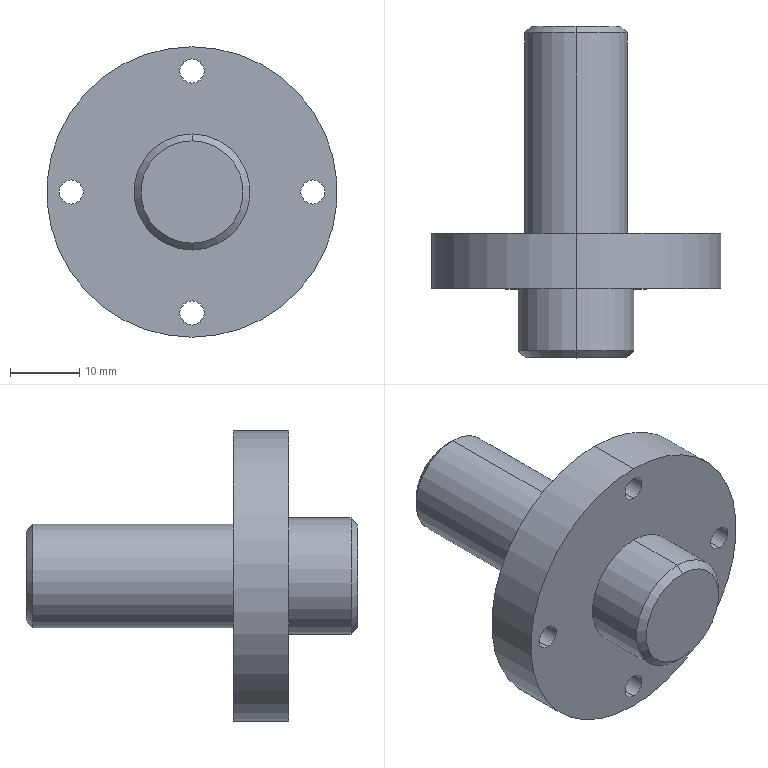Part | SolidWorks | features ICE 10, Chamfer 2, CirPattern 2, Extrusion 1 | 1 solid | 22 faces | box 42 x 48 x 42 mm | volume 18246 mm3 | cylinder 14 | cone 4 | plane 4 | commonest cylinder face diameters 3.5 x8 15 x2 16.8 x2 42 x2
STEP:
#1=CARTESIAN_POINT('',(0.,57.,-19.25));
#2=VERTEX_POINT('',#1);
#3=CARTESIAN_POINT('',(0.,57.,-15.75));
#4=VERTEX_POINT('',#3);
#5=CARTESIAN_POINT('',(0.,57.,-17.5));
#6=DIRECTION('',(0.,1.,0.));
#7=DIRECTION('',(0.,0.,1.));
#8=AXIS2_PLACEMENT_3D('',#5,#6,#7);
#9=CIRCLE('',#8,1.75);
#10=EDGE_CURVE('',#2,#4,#9,.T.);
#11=ORIENTED_EDGE('',*,*,#10,.F.);
#12=CARTESIAN_POINT('',(0.,65.,-19.25));
#13=VERTEX_POINT('',#12);
#14=CARTESIAN_POINT('',(0.,47.,-19.25));
#15=DIRECTION('',(0.,1.,0.));
#16=VECTOR('',#15,1000.);
#17=LINE('',#14,#16);
#18=EDGE_CURVE('',#2,#13,#17,.T.);
#19=ORIENTED_EDGE('',*,*,#18,.T.);
#20=CARTESIAN_POINT('',(0.,65.,-15.75));
#21=VERTEX_POINT('',#20);
#22=CARTESIAN_POINT('',(0.,65.,-17.5));
#23=DIRECTION('',(0.,1.,0.));
#24=DIRECTION('',(1.,0.,0.));
#25=AXIS2_PLACEMENT_3D('',#22,#23,#24);
#26=CIRCLE('',#25,1.75);
#27=EDGE_CURVE('',#13,#21,#26,.T.);
#28=ORIENTED_EDGE('',*,*,#27,.T.);
#29=CARTESIAN_POINT('',(0.,47.,-15.75));
#30=DIRECTION('',(0.,1.,0.));
#31=VECTOR('',#30,1000.);
#32=LINE('',#29,#31);
#33=EDGE_CURVE('',#4,#21,#32,.T.);
#34=ORIENTED_EDGE('',*,*,#33,.F.);
#35=EDGE_LOOP('',(#11,#19,#28,#34));
#36=FACE_OUTER_BOUND('',#35,.T.);
#37=CARTESIAN_POINT('',(0.,47.,-17.5));
#38=DIRECTION('',(0.,1.,0.));
#39=DIRECTION('',(0.,0.,1.));
#40=AXIS2_PLACEMENT_3D('',#37,#38,#39);
#41=CYLINDRICAL_SURFACE('',#40,1.75);
#42=ADVANCED_FACE('',(#36),#41,.F.);
#43=CARTESIAN_POINT('',(-17.5,57.,-1.75));
#44=VERTEX_POINT('',#43);
#45=CARTESIAN_POINT('',(-17.5,57.,1.75));
#46=VERTEX_POINT('',#45);
#47=CARTESIAN_POINT('',(-17.5,57.,0.));
#48=DIRECTION('',(0.,1.,0.));
#49=DIRECTION('',(0.,0.,1.));
#50=AXIS2_PLACEMENT_3D('',#47,#48,#49);
#51=CIRCLE('',#50,1.75);
#52=EDGE_CURVE('',#44,#46,#51,.T.);
#53=ORIENTED_EDGE('',*,*,#52,.F.);
#54=CARTESIAN_POINT('',(-17.5,65.,-1.75));
#55=VERTEX_POINT('',#54);
#56=CARTESIAN_POINT('',(-17.5,47.,-1.75));
#57=DIRECTION('',(0.,1.,0.));
#58=VECTOR('',#57,1000.);
#59=LINE('',#56,#58);
#60=EDGE_CURVE('',#44,#55,#59,.T.);
#61=ORIENTED_EDGE('',*,*,#60,.T.);
#62=CARTESIAN_POINT('',(-17.5,65.,1.75));
#63=VERTEX_POINT('',#62);
#64=CARTESIAN_POINT('',(-17.5,65.,0.));
#65=DIRECTION('',(0.,1.,0.));
#66=DIRECTION('',(0.,0.,-1.));
#67=AXIS2_PLACEMENT_3D('',#64,#65,#66);
#68=CIRCLE('',#67,1.75);
#69=EDGE_CURVE('',#55,#63,#68,.T.);
#70=ORIENTED_EDGE('',*,*,#69,.T.);
#71=CARTESIAN_POINT('',(-17.5,47.,1.75));
#72=DIRECTION('',(0.,1.,0.));
#73=VECTOR('',#72,1000.);
#74=LINE('',#71,#73);
#75=EDGE_CURVE('',#46,#63,#74,.T.);
#76=ORIENTED_EDGE('',*,*,#75,.F.);
#77=EDGE_LOOP('',(#53,#61,#70,#76));
#78=FACE_OUTER_BOUND('',#77,.T.);
#79=CARTESIAN_POINT('',(-17.5,47.,0.));
#80=DIRECTION('',(0.,1.,0.));
#81=DIRECTION('',(0.,0.,1.));
#82=AXIS2_PLACEMENT_3D('',#79,#80,#81);
#83=CYLINDRICAL_SURFACE('',#82,1.75);
#84=ADVANCED_FACE('',(#78),#83,.F.);
#85=CARTESIAN_POINT('',(0.,57.,15.75));
#86=VERTEX_POINT('',#85);
#87=CARTESIAN_POINT('',(0.,57.,19.25));
#88=VERTEX_POINT('',#87);
#89=CARTESIAN_POINT('',(0.,57.,17.5));
#90=DIRECTION('',(0.,1.,0.));
#91=DIRECTION('',(0.,0.,1.));
#92=AXIS2_PLACEMENT_3D('',#89,#90,#91);
#93=CIRCLE('',#92,1.75);
#94=EDGE_CURVE('',#86,#88,#93,.T.);
#95=ORIENTED_EDGE('',*,*,#94,.F.);
#96=CARTESIAN_POINT('',(0.,65.,15.75));
#97=VERTEX_POINT('',#96);
#98=CARTESIAN_POINT('',(0.,47.,15.75));
#99=DIRECTION('',(0.,1.,0.));
#100=VECTOR('',#99,1000.);
#101=LINE('',#98,#100);
#102=EDGE_CURVE('',#86,#97,#101,.T.);
#103=ORIENTED_EDGE('',*,*,#102,.T.);
#104=CARTESIAN_POINT('',(0.,65.,19.25));
#105=VERTEX_POINT('',#104);
#106=CARTESIAN_POINT('',(0.,65.,17.5));
#107=DIRECTION('',(0.,1.,0.));
#108=DIRECTION('',(-1.,0.,0.));
#109=AXIS2_PLACEMENT_3D('',#106,#107,#108);
#110=CIRCLE('',#109,1.75);
#111=EDGE_CURVE('',#97,#105,#110,.T.);
#112=ORIENTED_EDGE('',*,*,#111,.T.);
#113=CARTESIAN_POINT('',(0.,47.,19.25));
#114=DIRECTION('',(0.,1.,0.));
#115=VECTOR('',#114,1000.);
#116=LINE('',#113,#115);
#117=EDGE_CURVE('',#88,#105,#116,.T.);
#118=ORIENTED_EDGE('',*,*,#117,.F.);
#119=EDGE_LOOP('',(#95,#103,#112,#118));
#120=FACE_OUTER_BOUND('',#119,.T.);
#121=CARTESIAN_POINT('',(0.,47.,17.5));
#122=DIRECTION('',(0.,1.,0.));
#123=DIRECTION('',(0.,0.,1.));
#124=AXIS2_PLACEMENT_3D('',#121,#122,#123);
#125=CYLINDRICAL_SURFACE('',#124,1.75);
#126=ADVANCED_FACE('',(#120),#125,.F.);
#127=CARTESIAN_POINT('',(17.5,57.,-1.75));
#128=VERTEX_POINT('',#127);
#129=CARTESIAN_POINT('',(17.5,57.,1.75));
#130=VERTEX_POINT('',#129);
#131=CARTESIAN_POINT('',(17.5,57.,0.));
#132=DIRECTION('',(0.,1.,0.));
#133=DIRECTION('',(0.,0.,1.));
#134=AXIS2_PLACEMENT_3D('',#131,#132,#133);
#135=CIRCLE('',#134,1.75);
#136=EDGE_CURVE('',#128,#130,#135,.T.);
#137=ORIENTED_EDGE('',*,*,#136,.F.);
#138=CARTESIAN_POINT('',(17.5,65.,-1.75));
#139=VERTEX_POINT('',#138);
#140=CARTESIAN_POINT('',(17.5,47.,-1.75));
#141=DIRECTION('',(0.,1.,0.));
#142=VECTOR('',#141,1000.);
#143=LINE('',#140,#142);
#144=EDGE_CURVE('',#128,#139,#143,.T.);
#145=ORIENTED_EDGE('',*,*,#144,.T.);
#146=CARTESIAN_POINT('',(17.5,65.,1.75));
#147=VERTEX_POINT('',#146);
#148=CARTESIAN_POINT('',(17.5,65.,0.));
#149=DIRECTION('',(0.,1.,0.));
#150=DIRECTION('',(0.,0.,1.));
#151=AXIS2_PLACEMENT_3D('',#148,#149,#150);
#152=CIRCLE('',#151,1.75);
#153=EDGE_CURVE('',#139,#147,#152,.T.);
#154=ORIENTED_EDGE('',*,*,#153,.T.);
#155=CARTESIAN_POINT('',(17.5,47.,1.75));
#156=DIRECTION('',(0.,1.,0.));
#157=VECTOR('',#156,1000.);
#158=LINE('',#155,#157);
#159=EDGE_CURVE('',#130,#147,#158,.T.);
#160=ORIENTED_EDGE('',*,*,#159,.F.);
#161=EDGE_LOOP('',(#137,#145,#154,#160));
#162=FACE_OUTER_BOUND('',#161,.T.);
#163=CARTESIAN_POINT('',(17.5,47.,0.));
#164=DIRECTION('',(0.,1.,0.));
#165=DIRECTION('',(0.,0.,1.));
#166=AXIS2_PLACEMENT_3D('',#163,#164,#165);
#167=CYLINDRICAL_SURFACE('',#166,1.75);
#168=ADVANCED_FACE('',(#162),#167,.F.);
#169=CARTESIAN_POINT('',(0.,47.,-7.4));
#170=VERTEX_POINT('',#169);
#171=CARTESIAN_POINT('',(0.,47.,7.4));
#172=VERTEX_POINT('',#171);
#173=CARTESIAN_POINT('',(0.,47.,0.));
#174=DIRECTION('',(0.,-1.,0.));
#175=DIRECTION('',(0.,0.,-1.));
#176=AXIS2_PLACEMENT_3D('',#173,#174,#175);
#177=CIRCLE('',#176,7.4);
#178=EDGE_CURVE('',#170,#172,#177,.T.);
#179=ORIENTED_EDGE('',*,*,#178,.F.);
#180=CARTESIAN_POINT('',(0.,48.,-8.4));
#181=VERTEX_POINT('',#180);
#182=CARTESIAN_POINT('',(0.,47.,-7.4));
#183=DIRECTION('',(0.,0.7071,-0.7071));
#184=VECTOR('',#183,1000.);
#185=LINE('',#182,#184);
#186=EDGE_CURVE('',#170,#181,#185,.T.);
#187=ORIENTED_EDGE('',*,*,#186,.T.);
#188=CARTESIAN_POINT('',(0.,48.,8.4));
#189=VERTEX_POINT('',#188);
#190=CARTESIAN_POINT('',(0.,48.,0.));
#191=DIRECTION('',(0.,1.,0.));
#192=DIRECTION('',(0.,0.,-1.));
#193=AXIS2_PLACEMENT_3D('',#190,#191,#192);
#194=CIRCLE('',#193,8.4);
#195=EDGE_CURVE('',#189,#181,#194,.T.);
#196=ORIENTED_EDGE('',*,*,#195,.F.);
#197=CARTESIAN_POINT('',(0.,47.,7.4));
#198=DIRECTION('',(0.,0.7071,0.7071));
#199=VECTOR('',#198,1000.);
#200=LINE('',#197,#199);
#201=EDGE_CURVE('',#172,#189,#200,.T.);
#202=ORIENTED_EDGE('',*,*,#201,.F.);
#203=EDGE_LOOP('',(#179,#187,#196,#202));
#204=FACE_OUTER_BOUND('',#203,.T.);
#205=CARTESIAN_POINT('',(0.,47.,0.));
#206=DIRECTION('',(0.,1.,0.));
#207=DIRECTION('',(0.,0.,1.));
#208=AXIS2_PLACEMENT_3D('',#205,#206,#207);
#209=CONICAL_SURFACE('',#208,7.4,0.7854);
#210=ADVANCED_FACE('',(#204),#209,.T.);
#211=CARTESIAN_POINT('',(0.,95.,6.5));
#212=VERTEX_POINT('',#211);
#213=CARTESIAN_POINT('',(0.,95.,-6.5));
#214=VERTEX_POINT('',#213);
#215=CARTESIAN_POINT('',(0.,95.,0.));
#216=DIRECTION('',(0.,1.,0.));
#217=DIRECTION('',(0.,0.,1.));
#218=AXIS2_PLACEMENT_3D('',#215,#216,#217);
#219=CIRCLE('',#218,6.5);
#220=EDGE_CURVE('',#212,#214,#219,.T.);
#221=ORIENTED_EDGE('',*,*,#220,.F.);
#222=CARTESIAN_POINT('',(0.,94.,7.5));
#223=VERTEX_POINT('',#222);
#224=CARTESIAN_POINT('',(0.,95.,6.5));
#225=DIRECTION('',(0.,-0.7071,0.7071));
#226=VECTOR('',#225,1000.);
#227=LINE('',#224,#226);
#228=EDGE_CURVE('',#212,#223,#227,.T.);
#229=ORIENTED_EDGE('',*,*,#228,.T.);
#230=CARTESIAN_POINT('',(0.,94.,-7.5));
#231=VERTEX_POINT('',#230);
#232=CARTESIAN_POINT('',(0.,94.,0.));
#233=DIRECTION('',(0.,-1.,0.));
#234=DIRECTION('',(0.,0.,1.));
#235=AXIS2_PLACEMENT_3D('',#232,#233,#234);
#236=CIRCLE('',#235,7.5);
#237=EDGE_CURVE('',#231,#223,#236,.T.);
#238=ORIENTED_EDGE('',*,*,#237,.F.);
#239=CARTESIAN_POINT('',(0.,95.,-6.5));
#240=DIRECTION('',(0.,-0.7071,-0.7071));
#241=VECTOR('',#240,1000.);
#242=LINE('',#239,#241);
#243=EDGE_CURVE('',#214,#231,#242,.T.);
#244=ORIENTED_EDGE('',*,*,#243,.F.);
#245=EDGE_LOOP('',(#221,#229,#238,#244));
#246=FACE_OUTER_BOUND('',#245,.T.);
#247=CARTESIAN_POINT('',(0.,95.,0.));
#248=DIRECTION('',(0.,-1.,0.));
#249=DIRECTION('',(0.,0.,-1.));
#250=AXIS2_PLACEMENT_3D('',#247,#248,#249);
#251=CONICAL_SURFACE('',#250,6.5,0.7854);
#252=ADVANCED_FACE('',(#246),#251,.T.);
#253=ORIENTED_EDGE('',*,*,#195,.T.);
#254=CARTESIAN_POINT('',(0.,57.,-8.4));
#255=VERTEX_POINT('',#254);
#256=CARTESIAN_POINT('',(0.,47.,-8.4));
#257=DIRECTION('',(0.,1.,0.));
#258=VECTOR('',#257,1000.);
#259=LINE('',#256,#258);
#260=EDGE_CURVE('',#181,#255,#259,.T.);
#261=ORIENTED_EDGE('',*,*,#260,.T.);
#262=CARTESIAN_POINT('',(0.,57.,8.4));
#263=VERTEX_POINT('',#262);
#264=CARTESIAN_POINT('',(0.,57.,0.));
#265=DIRECTION('',(0.,-1.,0.));
#266=DIRECTION('',(0.,0.,1.));
#267=AXIS2_PLACEMENT_3D('',#264,#265,#266);
#268=CIRCLE('',#267,8.4);
#269=EDGE_CURVE('',#255,#263,#268,.T.);
#270=ORIENTED_EDGE('',*,*,#269,.T.);
#271=CARTESIAN_POINT('',(0.,47.,8.4));
#272=DIRECTION('',(0.,1.,0.));
#273=VECTOR('',#272,1000.);
#274=LINE('',#271,#273);
#275=EDGE_CURVE('',#189,#263,#274,.T.);
#276=ORIENTED_EDGE('',*,*,#275,.F.);
#277=EDGE_LOOP('',(#253,#261,#270,#276));
#278=FACE_OUTER_BOUND('',#277,.T.);
#279=CARTESIAN_POINT('',(0.,47.,0.));
#280=DIRECTION('',(0.,1.,0.));
#281=DIRECTION('',(0.,0.,1.));
#282=AXIS2_PLACEMENT_3D('',#279,#280,#281);
#283=CYLINDRICAL_SURFACE('',#282,8.4);
#284=ADVANCED_FACE('',(#278),#283,.T.);
#285=ORIENTED_EDGE('',*,*,#237,.T.);
#286=CARTESIAN_POINT('',(0.,65.,7.5));
#287=VERTEX_POINT('',#286);
#288=CARTESIAN_POINT('',(0.,95.,7.5));
#289=DIRECTION('',(0.,-1.,0.));
#290=VECTOR('',#289,1000.);
#291=LINE('',#288,#290);
#292=EDGE_CURVE('',#223,#287,#291,.T.);
#293=ORIENTED_EDGE('',*,*,#292,.T.);
#294=CARTESIAN_POINT('',(0.,65.,-7.5));
#295=VERTEX_POINT('',#294);
#296=CARTESIAN_POINT('',(0.,65.,0.));
#297=DIRECTION('',(0.,1.,0.));
#298=DIRECTION('',(0.,0.,1.));
#299=AXIS2_PLACEMENT_3D('',#296,#297,#298);
#300=CIRCLE('',#299,7.5);
#301=EDGE_CURVE('',#287,#295,#300,.T.);
#302=ORIENTED_EDGE('',*,*,#301,.T.);
#303=CARTESIAN_POINT('',(0.,95.,-7.5));
#304=DIRECTION('',(0.,-1.,0.));
#305=VECTOR('',#304,1000.);
#306=LINE('',#303,#305);
#307=EDGE_CURVE('',#231,#295,#306,.T.);
#308=ORIENTED_EDGE('',*,*,#307,.F.);
#309=EDGE_LOOP('',(#285,#293,#302,#308));
#310=FACE_OUTER_BOUND('',#309,.T.);
#311=CARTESIAN_POINT('',(0.,95.,0.));
#312=DIRECTION('',(0.,-1.,0.));
#313=DIRECTION('',(0.,0.,-1.));
#314=AXIS2_PLACEMENT_3D('',#311,#312,#313);
#315=CYLINDRICAL_SURFACE('',#314,7.5);
#316=ADVANCED_FACE('',(#310),#315,.T.);
#317=CARTESIAN_POINT('',(0.,57.,21.));
#318=VERTEX_POINT('',#317);
#319=CARTESIAN_POINT('',(0.,57.,-21.));
#320=VERTEX_POINT('',#319);
#321=CARTESIAN_POINT('',(0.,57.,0.));
#322=DIRECTION('',(0.,1.,0.));
#323=DIRECTION('',(0.,0.,1.));
#324=AXIS2_PLACEMENT_3D('',#321,#322,#323);
#325=CIRCLE('',#324,21.);
#326=EDGE_CURVE('',#318,#320,#325,.T.);
#327=ORIENTED_EDGE('',*,*,#326,.T.);
#328=CARTESIAN_POINT('',(0.,65.,-21.));
#329=VERTEX_POINT('',#328);
#330=CARTESIAN_POINT('',(0.,57.,-21.));
#331=DIRECTION('',(0.,1.,0.));
#332=VECTOR('',#331,1000.);
#333=LINE('',#330,#332);
#334=EDGE_CURVE('',#320,#329,#333,.T.);
#335=ORIENTED_EDGE('',*,*,#334,.T.);
#336=CARTESIAN_POINT('',(0.,65.,21.));
#337=VERTEX_POINT('',#336);
#338=CARTESIAN_POINT('',(0.,65.,0.));
#339=DIRECTION('',(0.,1.,0.));
#340=DIRECTION('',(0.,0.,1.));
#341=AXIS2_PLACEMENT_3D('',#338,#339,#340);
#342=CIRCLE('',#341,21.);
#343=EDGE_CURVE('',#337,#329,#342,.T.);
#344=ORIENTED_EDGE('',*,*,#343,.F.);
#345=CARTESIAN_POINT('',(0.,57.,21.));
#346=DIRECTION('',(0.,1.,0.));
#347=VECTOR('',#346,1000.);
#348=LINE('',#345,#347);
#349=EDGE_CURVE('',#318,#337,#348,.T.);
#350=ORIENTED_EDGE('',*,*,#349,.F.);
#351=EDGE_LOOP('',(#327,#335,#344,#350));
#352=FACE_OUTER_BOUND('',#351,.T.);
#353=CARTESIAN_POINT('',(0.,57.,0.));
#354=DIRECTION('',(0.,1.,0.));
#355=DIRECTION('',(0.,0.,1.));
#356=AXIS2_PLACEMENT_3D('',#353,#354,#355);
#357=CYLINDRICAL_SURFACE('',#356,21.);
#358=ADVANCED_FACE('',(#352),#357,.T.);
#359=CARTESIAN_POINT('',(0.,57.,-17.5));
#360=DIRECTION('',(0.,1.,0.));
#361=DIRECTION('',(0.,0.,1.));
#362=AXIS2_PLACEMENT_3D('',#359,#360,#361);
#363=CIRCLE('',#362,1.75);
#364=EDGE_CURVE('',#4,#2,#363,.T.);
#365=ORIENTED_EDGE('',*,*,#364,.T.);
#366=ORIENTED_EDGE('',*,*,#10,.T.);
#367=EDGE_LOOP('',(#365,#366));
#368=FACE_BOUND('',#367,.T.);
#369=CARTESIAN_POINT('',(-17.5,57.,0.));
#370=DIRECTION('',(0.,1.,0.));
#371=DIRECTION('',(0.,0.,1.));
#372=AXIS2_PLACEMENT_3D('',#369,#370,#371);
#373=CIRCLE('',#372,1.75);
#374=EDGE_CURVE('',#46,#44,#373,.T.);
#375=ORIENTED_EDGE('',*,*,#374,.T.);
#376=ORIENTED_EDGE('',*,*,#52,.T.);
#377=EDGE_LOOP('',(#375,#376));
#378=FACE_BOUND('',#377,.T.);
#379=CARTESIAN_POINT('',(0.,57.,17.5));
#380=DIRECTION('',(0.,1.,0.));
#381=DIRECTION('',(0.,0.,1.));
#382=AXIS2_PLACEMENT_3D('',#379,#380,#381);
#383=CIRCLE('',#382,1.75);
#384=EDGE_CURVE('',#88,#86,#383,.T.);
#385=ORIENTED_EDGE('',*,*,#384,.T.);
#386=ORIENTED_EDGE('',*,*,#94,.T.);
#387=EDGE_LOOP('',(#385,#386));
#388=FACE_BOUND('',#387,.T.);
#389=CARTESIAN_POINT('',(17.5,57.,0.));
#390=DIRECTION('',(0.,1.,0.));
#391=DIRECTION('',(0.,0.,1.));
#392=AXIS2_PLACEMENT_3D('',#389,#390,#391);
#393=CIRCLE('',#392,1.75);
#394=EDGE_CURVE('',#130,#128,#393,.T.);
#395=ORIENTED_EDGE('',*,*,#394,.T.);
#396=ORIENTED_EDGE('',*,*,#136,.T.);
#397=EDGE_LOOP('',(#395,#396));
#398=FACE_BOUND('',#397,.T.);
#399=ORIENTED_EDGE('',*,*,#326,.F.);
#400=CARTESIAN_POINT('',(0.,57.,0.));
#401=DIRECTION('',(0.,1.,0.));
#402=DIRECTION('',(0.,0.,1.));
#403=AXIS2_PLACEMENT_3D('',#400,#401,#402);
#404=CIRCLE('',#403,21.);
#405=EDGE_CURVE('',#320,#318,#404,.T.);
#406=ORIENTED_EDGE('',*,*,#405,.F.);
#407=EDGE_LOOP('',(#399,#406));
#408=FACE_OUTER_BOUND('',#407,.T.);
#409=CARTESIAN_POINT('',(0.,57.,0.));
#410=DIRECTION('',(0.,-1.,0.));
#411=DIRECTION('',(0.,0.,1.));
#412=AXIS2_PLACEMENT_3D('',#409,#410,#411);
#413=CIRCLE('',#412,8.4);
#414=EDGE_CURVE('',#263,#255,#413,.T.);
#415=ORIENTED_EDGE('',*,*,#414,.F.);
#416=ORIENTED_EDGE('',*,*,#269,.F.);
#417=EDGE_LOOP('',(#415,#416));
#418=FACE_BOUND('',#417,.T.);
#419=CARTESIAN_POINT('',(0.,57.,0.));
#420=DIRECTION('',(0.,1.,0.));
#421=DIRECTION('',(0.,0.,1.));
#422=AXIS2_PLACEMENT_3D('',#419,#420,#421);
#423=PLANE('',#422);
#424=ADVANCED_FACE('',(#368,#378,#388,#398,#408,#418),#423,.F.);
#425=ORIENTED_EDGE('',*,*,#334,.F.);
#426=ORIENTED_EDGE('',*,*,#405,.T.);
#427=ORIENTED_EDGE('',*,*,#349,.T.);
#428=CARTESIAN_POINT('',(0.,65.,0.));
#429=DIRECTION('',(0.,1.,0.));
#430=DIRECTION('',(0.,0.,1.));
#431=AXIS2_PLACEMENT_3D('',#428,#429,#430);
#432=CIRCLE('',#431,21.);
#433=EDGE_CURVE('',#329,#337,#432,.T.);
#434=ORIENTED_EDGE('',*,*,#433,.F.);
#435=EDGE_LOOP('',(#425,#426,#427,#434));
#436=FACE_OUTER_BOUND('',#435,.T.);
#437=CARTESIAN_POINT('',(0.,57.,0.));
#438=DIRECTION('',(0.,1.,0.));
#439=DIRECTION('',(0.,0.,1.));
#440=AXIS2_PLACEMENT_3D('',#437,#438,#439);
#441=CYLINDRICAL_SURFACE('',#440,21.);
#442=ADVANCED_FACE('',(#436),#441,.T.);
#443=CARTESIAN_POINT('',(0.,95.,0.));
#444=DIRECTION('',(0.,1.,0.));
#445=DIRECTION('',(0.,0.,1.));
#446=AXIS2_PLACEMENT_3D('',#443,#444,#445);
#447=CIRCLE('',#446,6.5);
#448=EDGE_CURVE('',#214,#212,#447,.T.);
#449=ORIENTED_EDGE('',*,*,#448,.T.);
#450=ORIENTED_EDGE('',*,*,#220,.T.);
#451=EDGE_LOOP('',(#449,#450));
#452=FACE_OUTER_BOUND('',#451,.T.);
#453=CARTESIAN_POINT('',(0.,95.,0.));
#454=DIRECTION('',(0.,1.,0.));
#455=DIRECTION('',(0.,0.,1.));
#456=AXIS2_PLACEMENT_3D('',#453,#454,#455);
#457=PLANE('',#456);
#458=ADVANCED_FACE('',(#452),#457,.T.);
#459=ORIENTED_EDGE('',*,*,#292,.F.);
#460=CARTESIAN_POINT('',(0.,94.,0.));
#461=DIRECTION('',(0.,-1.,0.));
#462=DIRECTION('',(0.,0.,1.));
#463=AXIS2_PLACEMENT_3D('',#460,#461,#462);
#464=CIRCLE('',#463,7.5);
#465=EDGE_CURVE('',#223,#231,#464,.T.);
#466=ORIENTED_EDGE('',*,*,#465,.T.);
#467=ORIENTED_EDGE('',*,*,#307,.T.);
#468=CARTESIAN_POINT('',(0.,65.,0.));
#469=DIRECTION('',(0.,1.,0.));
#470=DIRECTION('',(0.,0.,1.));
#471=AXIS2_PLACEMENT_3D('',#468,#469,#470);
#472=CIRCLE('',#471,7.5);
#473=EDGE_CURVE('',#295,#287,#472,.T.);
#474=ORIENTED_EDGE('',*,*,#473,.T.);
#475=EDGE_LOOP('',(#459,#466,#467,#474));
#476=FACE_OUTER_BOUND('',#475,.T.);
#477=CARTESIAN_POINT('',(0.,95.,0.));
#478=DIRECTION('',(0.,-1.,0.));
#479=DIRECTION('',(0.,0.,-1.));
#480=AXIS2_PLACEMENT_3D('',#477,#478,#479);
#481=CYLINDRICAL_SURFACE('',#480,7.5);
#482=ADVANCED_FACE('',(#476),#481,.T.);
#483=CARTESIAN_POINT('',(0.,65.,-17.5));
#484=DIRECTION('',(0.,1.,0.));
#485=DIRECTION('',(1.,0.,0.));
#486=AXIS2_PLACEMENT_3D('',#483,#484,#485);
#487=CIRCLE('',#486,1.75);
#488=EDGE_CURVE('',#21,#13,#487,.T.);
#489=ORIENTED_EDGE('',*,*,#488,.F.);
#490=ORIENTED_EDGE('',*,*,#27,.F.);
#491=EDGE_LOOP('',(#489,#490));
#492=FACE_BOUND('',#491,.T.);
#493=CARTESIAN_POINT('',(-17.5,65.,0.));
#494=DIRECTION('',(0.,1.,0.));
#495=DIRECTION('',(0.,0.,-1.));
#496=AXIS2_PLACEMENT_3D('',#493,#494,#495);
#497=CIRCLE('',#496,1.75);
#498=EDGE_CURVE('',#63,#55,#497,.T.);
#499=ORIENTED_EDGE('',*,*,#498,.F.);
#500=ORIENTED_EDGE('',*,*,#69,.F.);
#501=EDGE_LOOP('',(#499,#500));
#502=FACE_BOUND('',#501,.T.);
#503=CARTESIAN_POINT('',(0.,65.,17.5));
#504=DIRECTION('',(0.,1.,0.));
#505=DIRECTION('',(-1.,0.,0.));
#506=AXIS2_PLACEMENT_3D('',#503,#504,#505);
#507=CIRCLE('',#506,1.75);
#508=EDGE_CURVE('',#105,#97,#507,.T.);
#509=ORIENTED_EDGE('',*,*,#508,.F.);
#510=ORIENTED_EDGE('',*,*,#111,.F.);
#511=EDGE_LOOP('',(#509,#510));
#512=FACE_BOUND('',#511,.T.);
#513=CARTESIAN_POINT('',(17.5,65.,0.));
#514=DIRECTION('',(0.,1.,0.));
#515=DIRECTION('',(0.,0.,1.));
#516=AXIS2_PLACEMENT_3D('',#513,#514,#515);
#517=CIRCLE('',#516,1.75);
#518=EDGE_CURVE('',#147,#139,#517,.T.);
#519=ORIENTED_EDGE('',*,*,#518,.F.);
#520=ORIENTED_EDGE('',*,*,#153,.F.);
#521=EDGE_LOOP('',(#519,#520));
#522=FACE_BOUND('',#521,.T.);
#523=ORIENTED_EDGE('',*,*,#473,.F.);
#524=ORIENTED_EDGE('',*,*,#301,.F.);
#525=EDGE_LOOP('',(#523,#524));
#526=FACE_BOUND('',#525,.T.);
#527=ORIENTED_EDGE('',*,*,#343,.T.);
#528=ORIENTED_EDGE('',*,*,#433,.T.);
#529=EDGE_LOOP('',(#527,#528));
#530=FACE_OUTER_BOUND('',#529,.T.);
#531=CARTESIAN_POINT('',(0.,65.,0.));
#532=DIRECTION('',(0.,1.,0.));
#533=DIRECTION('',(0.,0.,1.));
#534=AXIS2_PLACEMENT_3D('',#531,#532,#533);
#535=PLANE('',#534);
#536=ADVANCED_FACE('',(#492,#502,#512,#522,#526,#530),#535,.T.);
#537=ORIENTED_EDGE('',*,*,#260,.F.);
#538=CARTESIAN_POINT('',(0.,48.,0.));
#539=DIRECTION('',(0.,1.,0.));
#540=DIRECTION('',(0.,0.,-1.));
#541=AXIS2_PLACEMENT_3D('',#538,#539,#540);
#542=CIRCLE('',#541,8.4);
#543=EDGE_CURVE('',#181,#189,#542,.T.);
#544=ORIENTED_EDGE('',*,*,#543,.T.);
#545=ORIENTED_EDGE('',*,*,#275,.T.);
#546=ORIENTED_EDGE('',*,*,#414,.T.);
#547=EDGE_LOOP('',(#537,#544,#545,#546));
#548=FACE_OUTER_BOUND('',#547,.T.);
#549=CARTESIAN_POINT('',(0.,47.,0.));
#550=DIRECTION('',(0.,1.,0.));
#551=DIRECTION('',(0.,0.,1.));
#552=AXIS2_PLACEMENT_3D('',#549,#550,#551);
#553=CYLINDRICAL_SURFACE('',#552,8.4);
#554=ADVANCED_FACE('',(#548),#553,.T.);
#555=CARTESIAN_POINT('',(0.,47.,0.));
#556=DIRECTION('',(0.,-1.,0.));
#557=DIRECTION('',(0.,0.,-1.));
#558=AXIS2_PLACEMENT_3D('',#555,#556,#557);
#559=CIRCLE('',#558,7.4);
#560=EDGE_CURVE('',#172,#170,#559,.T.);
#561=ORIENTED_EDGE('',*,*,#560,.T.);
#562=ORIENTED_EDGE('',*,*,#178,.T.);
#563=EDGE_LOOP('',(#561,#562));
#564=FACE_OUTER_BOUND('',#563,.T.);
#565=CARTESIAN_POINT('',(0.,47.,0.));
#566=DIRECTION('',(0.,-1.,0.));
#567=DIRECTION('',(0.,0.,-1.));
#568=AXIS2_PLACEMENT_3D('',#565,#566,#567);
#569=PLANE('',#568);
#570=ADVANCED_FACE('',(#564),#569,.T.);
#571=ORIENTED_EDGE('',*,*,#228,.F.);
#572=ORIENTED_EDGE('',*,*,#448,.F.);
#573=ORIENTED_EDGE('',*,*,#243,.T.);
#574=ORIENTED_EDGE('',*,*,#465,.F.);
#575=EDGE_LOOP('',(#571,#572,#573,#574));
#576=FACE_OUTER_BOUND('',#575,.T.);
#577=CARTESIAN_POINT('',(0.,95.,0.));
#578=DIRECTION('',(0.,-1.,0.));
#579=DIRECTION('',(0.,0.,-1.));
#580=AXIS2_PLACEMENT_3D('',#577,#578,#579);
#581=CONICAL_SURFACE('',#580,6.5,0.7854);
#582=ADVANCED_FACE('',(#576),#581,.T.);
#583=ORIENTED_EDGE('',*,*,#186,.F.);
#584=ORIENTED_EDGE('',*,*,#560,.F.);
#585=ORIENTED_EDGE('',*,*,#201,.T.);
#586=ORIENTED_EDGE('',*,*,#543,.F.);
#587=EDGE_LOOP('',(#583,#584,#585,#586));
#588=FACE_OUTER_BOUND('',#587,.T.);
#589=CARTESIAN_POINT('',(0.,47.,0.));
#590=DIRECTION('',(0.,1.,0.));
#591=DIRECTION('',(0.,0.,1.));
#592=AXIS2_PLACEMENT_3D('',#589,#590,#591);
#593=CONICAL_SURFACE('',#592,7.4,0.7854);
#594=ADVANCED_FACE('',(#588),#593,.T.);
#595=ORIENTED_EDGE('',*,*,#144,.F.);
#596=ORIENTED_EDGE('',*,*,#394,.F.);
#597=ORIENTED_EDGE('',*,*,#159,.T.);
#598=ORIENTED_EDGE('',*,*,#518,.T.);
#599=EDGE_LOOP('',(#595,#596,#597,#598));
#600=FACE_OUTER_BOUND('',#599,.T.);
#601=CARTESIAN_POINT('',(17.5,47.,0.));
#602=DIRECTION('',(0.,1.,0.));
#603=DIRECTION('',(0.,0.,1.));
#604=AXIS2_PLACEMENT_3D('',#601,#602,#603);
#605=CYLINDRICAL_SURFACE('',#604,1.75);
#606=ADVANCED_FACE('',(#600),#605,.F.);
#607=ORIENTED_EDGE('',*,*,#102,.F.);
#608=ORIENTED_EDGE('',*,*,#384,.F.);
#609=ORIENTED_EDGE('',*,*,#117,.T.);
#610=ORIENTED_EDGE('',*,*,#508,.T.);
#611=EDGE_LOOP('',(#607,#608,#609,#610));
#612=FACE_OUTER_BOUND('',#611,.T.);
#613=CARTESIAN_POINT('',(0.,47.,17.5));
#614=DIRECTION('',(0.,1.,0.));
#615=DIRECTION('',(0.,0.,1.));
#616=AXIS2_PLACEMENT_3D('',#613,#614,#615);
#617=CYLINDRICAL_SURFACE('',#616,1.75);
#618=ADVANCED_FACE('',(#612),#617,.F.);
#619=ORIENTED_EDGE('',*,*,#60,.F.);
#620=ORIENTED_EDGE('',*,*,#374,.F.);
#621=ORIENTED_EDGE('',*,*,#75,.T.);
#622=ORIENTED_EDGE('',*,*,#498,.T.);
#623=EDGE_LOOP('',(#619,#620,#621,#622));
#624=FACE_OUTER_BOUND('',#623,.T.);
#625=CARTESIAN_POINT('',(-17.5,47.,0.));
#626=DIRECTION('',(0.,1.,0.));
#627=DIRECTION('',(0.,0.,1.));
#628=AXIS2_PLACEMENT_3D('',#625,#626,#627);
#629=CYLINDRICAL_SURFACE('',#628,1.75);
#630=ADVANCED_FACE('',(#624),#629,.F.);
#631=ORIENTED_EDGE('',*,*,#18,.F.);
#632=ORIENTED_EDGE('',*,*,#364,.F.);
#633=ORIENTED_EDGE('',*,*,#33,.T.);
#634=ORIENTED_EDGE('',*,*,#488,.T.);
#635=EDGE_LOOP('',(#631,#632,#633,#634));
#636=FACE_OUTER_BOUND('',#635,.T.);
#637=CARTESIAN_POINT('',(0.,47.,-17.5));
#638=DIRECTION('',(0.,1.,0.));
#639=DIRECTION('',(0.,0.,1.));
#640=AXIS2_PLACEMENT_3D('',#637,#638,#639);
#641=CYLINDRICAL_SURFACE('',#640,1.75);
#642=ADVANCED_FACE('',(#636),#641,.F.);
#643=CLOSED_SHELL('',(#42,#84,#126,#168,#210,#252,#284,#316,#358,#424,#442,#458,#482,#536,#554,#570,#582,#594,#606,#618,#630,#642));
#644=MANIFOLD_SOLID_BREP('',#643);
#645=CARTESIAN_POINT('',(0.,0.,0.));
#646=DIRECTION('',(0.,0.,1.));
#647=DIRECTION('',(1.,0.,0.));
#648=AXIS2_PLACEMENT_3D('',#645,#646,#647);
#649=(LENGTH_UNIT()NAMED_UNIT(*)SI_UNIT(.MILLI.,.METRE.));
#650=UNCERTAINTY_MEASURE_WITH_UNIT(LENGTH_MEASURE(0.00001),#649,'','');
#651=(NAMED_UNIT(*)PLANE_ANGLE_UNIT()SI_UNIT($,.RADIAN.));
#652=(NAMED_UNIT(*)SI_UNIT($,.STERADIAN.)SOLID_ANGLE_UNIT());
#653=(GEOMETRIC_REPRESENTATION_CONTEXT(3)GLOBAL_UNCERTAINTY_ASSIGNED_CONTEXT((#650))GLOBAL_UNIT_ASSIGNED_CONTEXT((#649,#651,#652))REPRESENTATION_CONTEXT('',''));
#654=ADVANCED_BREP_SHAPE_REPRESENTATION('',(#644,#648),#653);